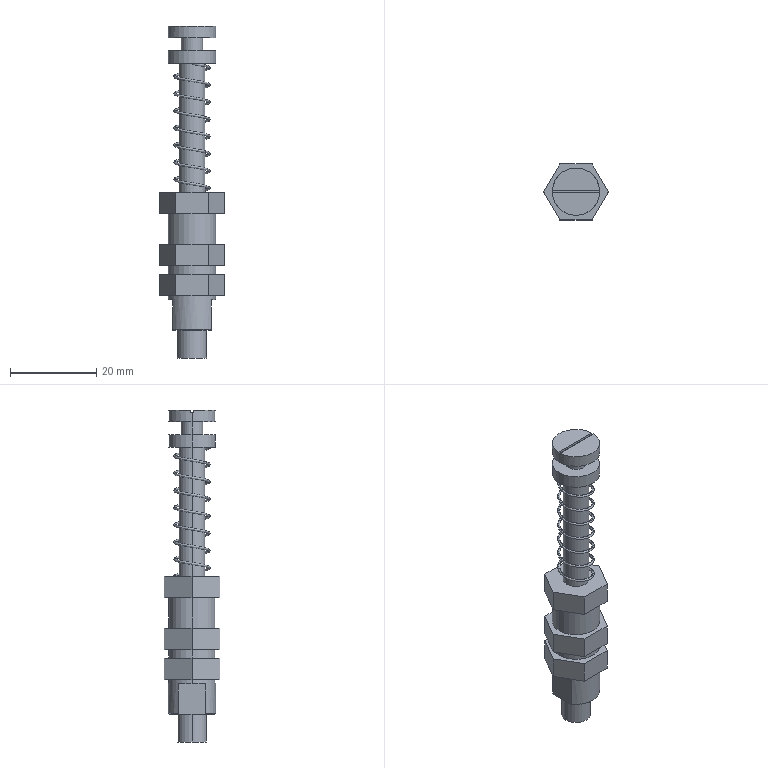Part | STEP file | PJ90 | 1 solid | 60 faces | box 15.011 x 13 x 77.2 mm | volume 5466 mm3 | plane 40 | cylinder 16 | spline 2 | cone 2 | commonest cylinder face diameters 11 x10 5 x2 6 x2 6.748 x2